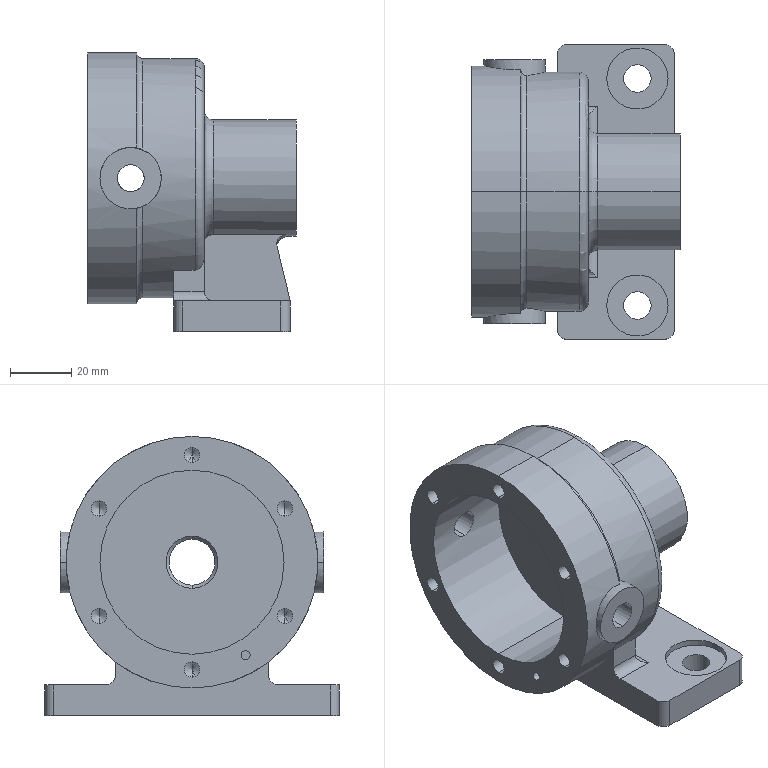Part | SolidWorks | features ICE 7, HoleWzd 4, Revolution 2, Chamfer 1, Fillet 1, Rib 1 | 1 solid | 106 faces | box 68 x 96 x 91 mm | volume 170738 mm3 | cylinder 56 | plane 22 | cone 20 | torus 7 | spline 1 | commonest cylinder face diameters 5 x12 6 x8 20 x8 3.3 x6 8.8 x4 9 x4